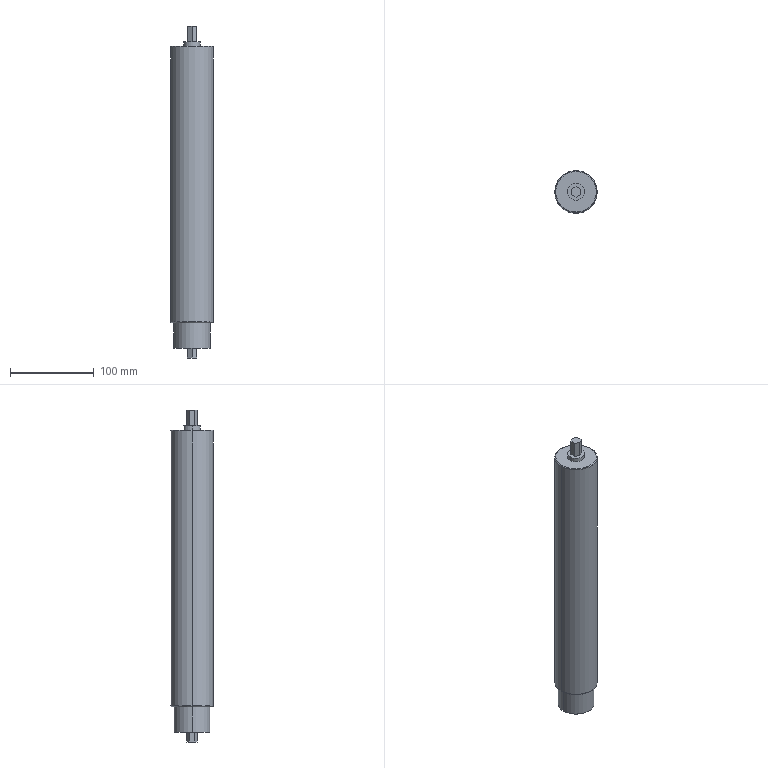Part | STEP file | Unpowered Roller_Default | 1 solid | 28 faces | box 50.6 x 50.6 x 396 mm | volume 712589 mm3 | plane 18 | cylinder 6 | torus 4 | commonest cylinder face diameters 20 x2 43 x2 50.6 x2